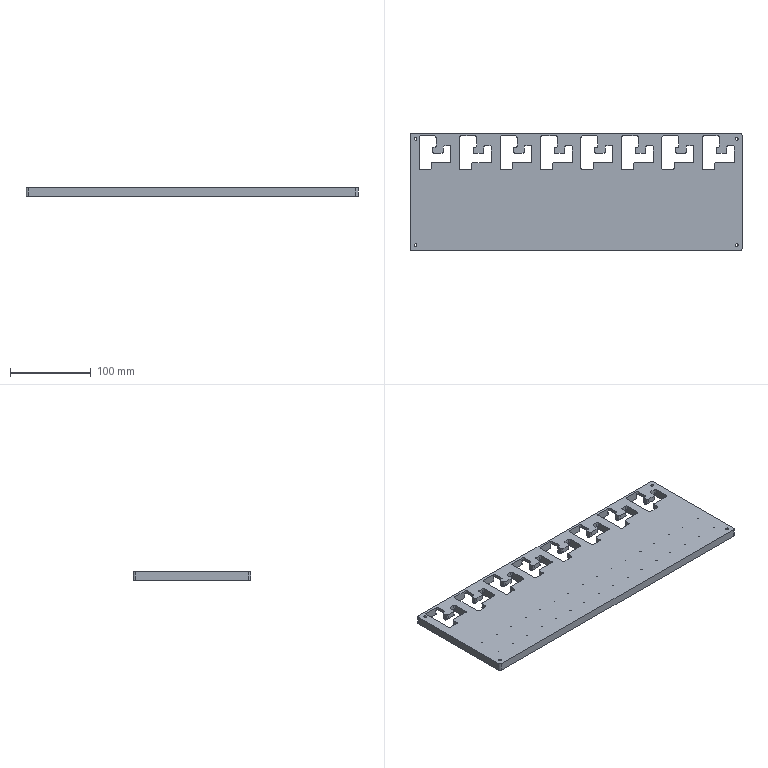Part | 1 solid | 2062 faces | box 410 x 145 x 10 mm | volume 382913 mm3 | plane 994 | cylinder 956 | cone 112 | commonest cylinder face diameters 2.5 x279 3.5 x200 1.5 x96 1.6 x80 0.5 x72 3.2 x56